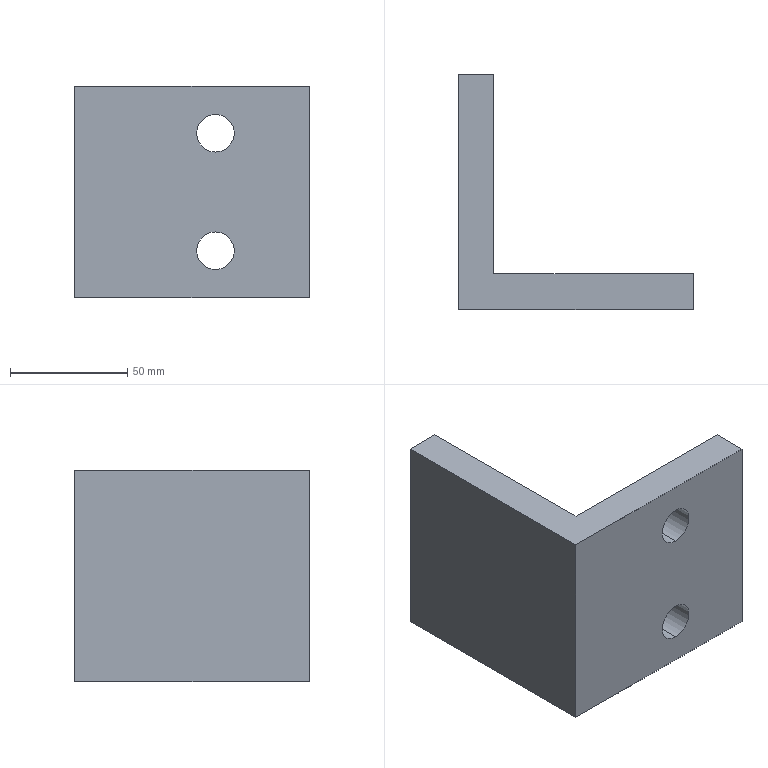Part | SolidWorks | features Extrusion 1, ICE 1 | 1 solid | 12 faces | box 100 x 100 x 90 mm | volume 243718 mm3 | plane 8 | cylinder 4 | commonest cylinder face diameters 16 x4
STEP:
#1=CARTESIAN_POINT('',(60.,0.,12.));
#2=VERTEX_POINT('',#1);
#3=CARTESIAN_POINT('',(60.,0.,28.));
#4=VERTEX_POINT('',#3);
#5=CARTESIAN_POINT('',(60.,0.,20.));
#6=DIRECTION('',(0.,1.,0.));
#7=DIRECTION('',(0.,0.,1.));
#8=AXIS2_PLACEMENT_3D('',#5,#6,#7);
#9=CIRCLE('',#8,8.);
#10=EDGE_CURVE('',#2,#4,#9,.T.);
#11=ORIENTED_EDGE('',*,*,#10,.F.);
#12=CARTESIAN_POINT('',(60.,15.,12.));
#13=VERTEX_POINT('',#12);
#14=CARTESIAN_POINT('',(60.,-75.,12.));
#15=DIRECTION('',(0.,1.,0.));
#16=VECTOR('',#15,1000.);
#17=LINE('',#14,#16);
#18=EDGE_CURVE('',#2,#13,#17,.T.);
#19=ORIENTED_EDGE('',*,*,#18,.T.);
#20=CARTESIAN_POINT('',(60.,15.,28.));
#21=VERTEX_POINT('',#20);
#22=CARTESIAN_POINT('',(60.,15.,20.));
#23=DIRECTION('',(0.,1.,0.));
#24=DIRECTION('',(0.,0.,1.));
#25=AXIS2_PLACEMENT_3D('',#22,#23,#24);
#26=CIRCLE('',#25,8.);
#27=EDGE_CURVE('',#13,#21,#26,.T.);
#28=ORIENTED_EDGE('',*,*,#27,.T.);
#29=CARTESIAN_POINT('',(60.,-75.,28.));
#30=DIRECTION('',(0.,1.,0.));
#31=VECTOR('',#30,1000.);
#32=LINE('',#29,#31);
#33=EDGE_CURVE('',#4,#21,#32,.T.);
#34=ORIENTED_EDGE('',*,*,#33,.F.);
#35=EDGE_LOOP('',(#11,#19,#28,#34));
#36=FACE_OUTER_BOUND('',#35,.T.);
#37=CARTESIAN_POINT('',(60.,-75.,20.));
#38=DIRECTION('',(0.,1.,0.));
#39=DIRECTION('',(0.,0.,1.));
#40=AXIS2_PLACEMENT_3D('',#37,#38,#39);
#41=CYLINDRICAL_SURFACE('',#40,8.);
#42=ADVANCED_FACE('',(#36),#41,.F.);
#43=CARTESIAN_POINT('',(60.,0.,62.));
#44=VERTEX_POINT('',#43);
#45=CARTESIAN_POINT('',(60.,0.,78.));
#46=VERTEX_POINT('',#45);
#47=CARTESIAN_POINT('',(60.,0.,70.));
#48=DIRECTION('',(0.,1.,0.));
#49=DIRECTION('',(0.,0.,1.));
#50=AXIS2_PLACEMENT_3D('',#47,#48,#49);
#51=CIRCLE('',#50,8.);
#52=EDGE_CURVE('',#44,#46,#51,.T.);
#53=ORIENTED_EDGE('',*,*,#52,.F.);
#54=CARTESIAN_POINT('',(60.,15.,62.));
#55=VERTEX_POINT('',#54);
#56=CARTESIAN_POINT('',(60.,-75.,62.));
#57=DIRECTION('',(0.,1.,0.));
#58=VECTOR('',#57,1000.);
#59=LINE('',#56,#58);
#60=EDGE_CURVE('',#44,#55,#59,.T.);
#61=ORIENTED_EDGE('',*,*,#60,.T.);
#62=CARTESIAN_POINT('',(60.,15.,78.));
#63=VERTEX_POINT('',#62);
#64=CARTESIAN_POINT('',(60.,15.,70.));
#65=DIRECTION('',(0.,1.,0.));
#66=DIRECTION('',(0.,0.,1.));
#67=AXIS2_PLACEMENT_3D('',#64,#65,#66);
#68=CIRCLE('',#67,8.);
#69=EDGE_CURVE('',#55,#63,#68,.T.);
#70=ORIENTED_EDGE('',*,*,#69,.T.);
#71=CARTESIAN_POINT('',(60.,-75.,78.));
#72=DIRECTION('',(0.,1.,0.));
#73=VECTOR('',#72,1000.);
#74=LINE('',#71,#73);
#75=EDGE_CURVE('',#46,#63,#74,.T.);
#76=ORIENTED_EDGE('',*,*,#75,.F.);
#77=EDGE_LOOP('',(#53,#61,#70,#76));
#78=FACE_OUTER_BOUND('',#77,.T.);
#79=CARTESIAN_POINT('',(60.,-75.,70.));
#80=DIRECTION('',(0.,1.,0.));
#81=DIRECTION('',(0.,0.,1.));
#82=AXIS2_PLACEMENT_3D('',#79,#80,#81);
#83=CYLINDRICAL_SURFACE('',#82,8.);
#84=ADVANCED_FACE('',(#78),#83,.F.);
#85=CARTESIAN_POINT('',(60.,0.,20.));
#86=DIRECTION('',(0.,1.,0.));
#87=DIRECTION('',(0.,0.,1.));
#88=AXIS2_PLACEMENT_3D('',#85,#86,#87);
#89=CIRCLE('',#88,8.);
#90=EDGE_CURVE('',#4,#2,#89,.T.);
#91=ORIENTED_EDGE('',*,*,#90,.T.);
#92=ORIENTED_EDGE('',*,*,#10,.T.);
#93=EDGE_LOOP('',(#91,#92));
#94=FACE_BOUND('',#93,.T.);
#95=CARTESIAN_POINT('',(60.,0.,70.));
#96=DIRECTION('',(0.,1.,0.));
#97=DIRECTION('',(0.,0.,1.));
#98=AXIS2_PLACEMENT_3D('',#95,#96,#97);
#99=CIRCLE('',#98,8.);
#100=EDGE_CURVE('',#46,#44,#99,.T.);
#101=ORIENTED_EDGE('',*,*,#100,.T.);
#102=ORIENTED_EDGE('',*,*,#52,.T.);
#103=EDGE_LOOP('',(#101,#102));
#104=FACE_BOUND('',#103,.T.);
#105=CARTESIAN_POINT('',(0.,0.,0.));
#106=VERTEX_POINT('',#105);
#107=CARTESIAN_POINT('',(100.,0.,0.));
#108=VERTEX_POINT('',#107);
#109=CARTESIAN_POINT('',(100.,0.,0.));
#110=DIRECTION('',(1.,0.,0.));
#111=VECTOR('',#110,1000.);
#112=LINE('',#109,#111);
#113=EDGE_CURVE('',#106,#108,#112,.T.);
#114=ORIENTED_EDGE('',*,*,#113,.T.);
#115=CARTESIAN_POINT('',(100.,0.,90.));
#116=VERTEX_POINT('',#115);
#117=CARTESIAN_POINT('',(100.,0.,90.));
#118=DIRECTION('',(0.,0.,-1.));
#119=VECTOR('',#118,1000.);
#120=LINE('',#117,#119);
#121=EDGE_CURVE('',#116,#108,#120,.T.);
#122=ORIENTED_EDGE('',*,*,#121,.F.);
#123=CARTESIAN_POINT('',(0.,0.,90.));
#124=VERTEX_POINT('',#123);
#125=CARTESIAN_POINT('',(100.,0.,90.));
#126=DIRECTION('',(1.,0.,0.));
#127=VECTOR('',#126,1000.);
#128=LINE('',#125,#127);
#129=EDGE_CURVE('',#124,#116,#128,.T.);
#130=ORIENTED_EDGE('',*,*,#129,.F.);
#131=CARTESIAN_POINT('',(0.,0.,90.));
#132=DIRECTION('',(0.,0.,-1.));
#133=VECTOR('',#132,1000.);
#134=LINE('',#131,#133);
#135=EDGE_CURVE('',#124,#106,#134,.T.);
#136=ORIENTED_EDGE('',*,*,#135,.T.);
#137=EDGE_LOOP('',(#114,#122,#130,#136));
#138=FACE_OUTER_BOUND('',#137,.T.);
#139=CARTESIAN_POINT('',(100.,0.,90.));
#140=DIRECTION('',(0.,1.,0.));
#141=DIRECTION('',(0.,0.,1.));
#142=AXIS2_PLACEMENT_3D('',#139,#140,#141);
#143=PLANE('',#142);
#144=ADVANCED_FACE('',(#94,#104,#138),#143,.F.);
#145=CARTESIAN_POINT('',(100.,15.,0.));
#146=VERTEX_POINT('',#145);
#147=CARTESIAN_POINT('',(100.,15.,0.));
#148=DIRECTION('',(0.,1.,0.));
#149=VECTOR('',#148,1000.);
#150=LINE('',#147,#149);
#151=EDGE_CURVE('',#108,#146,#150,.T.);
#152=ORIENTED_EDGE('',*,*,#151,.T.);
#153=CARTESIAN_POINT('',(100.,15.,90.));
#154=VERTEX_POINT('',#153);
#155=CARTESIAN_POINT('',(100.,15.,90.));
#156=DIRECTION('',(0.,0.,-1.));
#157=VECTOR('',#156,1000.);
#158=LINE('',#155,#157);
#159=EDGE_CURVE('',#154,#146,#158,.T.);
#160=ORIENTED_EDGE('',*,*,#159,.F.);
#161=CARTESIAN_POINT('',(100.,15.,90.));
#162=DIRECTION('',(0.,1.,0.));
#163=VECTOR('',#162,1000.);
#164=LINE('',#161,#163);
#165=EDGE_CURVE('',#116,#154,#164,.T.);
#166=ORIENTED_EDGE('',*,*,#165,.F.);
#167=ORIENTED_EDGE('',*,*,#121,.T.);
#168=EDGE_LOOP('',(#152,#160,#166,#167));
#169=FACE_OUTER_BOUND('',#168,.T.);
#170=CARTESIAN_POINT('',(100.,15.,90.));
#171=DIRECTION('',(-1.,0.,0.));
#172=DIRECTION('',(0.,0.,1.));
#173=AXIS2_PLACEMENT_3D('',#170,#171,#172);
#174=PLANE('',#173);
#175=ADVANCED_FACE('',(#169),#174,.F.);
#176=CARTESIAN_POINT('',(60.,15.,20.));
#177=DIRECTION('',(0.,1.,0.));
#178=DIRECTION('',(0.,0.,1.));
#179=AXIS2_PLACEMENT_3D('',#176,#177,#178);
#180=CIRCLE('',#179,8.);
#181=EDGE_CURVE('',#21,#13,#180,.T.);
#182=ORIENTED_EDGE('',*,*,#181,.F.);
#183=ORIENTED_EDGE('',*,*,#27,.F.);
#184=EDGE_LOOP('',(#182,#183));
#185=FACE_BOUND('',#184,.T.);
#186=CARTESIAN_POINT('',(60.,15.,70.));
#187=DIRECTION('',(0.,1.,0.));
#188=DIRECTION('',(0.,0.,1.));
#189=AXIS2_PLACEMENT_3D('',#186,#187,#188);
#190=CIRCLE('',#189,8.);
#191=EDGE_CURVE('',#63,#55,#190,.T.);
#192=ORIENTED_EDGE('',*,*,#191,.F.);
#193=ORIENTED_EDGE('',*,*,#69,.F.);
#194=EDGE_LOOP('',(#192,#193));
#195=FACE_BOUND('',#194,.T.);
#196=CARTESIAN_POINT('',(15.,15.,0.));
#197=VERTEX_POINT('',#196);
#198=CARTESIAN_POINT('',(15.,15.,0.));
#199=DIRECTION('',(-1.,0.,0.));
#200=VECTOR('',#199,1000.);
#201=LINE('',#198,#200);
#202=EDGE_CURVE('',#146,#197,#201,.T.);
#203=ORIENTED_EDGE('',*,*,#202,.T.);
#204=CARTESIAN_POINT('',(15.,15.,90.));
#205=VERTEX_POINT('',#204);
#206=CARTESIAN_POINT('',(15.,15.,90.));
#207=DIRECTION('',(0.,0.,-1.));
#208=VECTOR('',#207,1000.);
#209=LINE('',#206,#208);
#210=EDGE_CURVE('',#205,#197,#209,.T.);
#211=ORIENTED_EDGE('',*,*,#210,.F.);
#212=CARTESIAN_POINT('',(15.,15.,90.));
#213=DIRECTION('',(-1.,0.,0.));
#214=VECTOR('',#213,1000.);
#215=LINE('',#212,#214);
#216=EDGE_CURVE('',#154,#205,#215,.T.);
#217=ORIENTED_EDGE('',*,*,#216,.F.);
#218=ORIENTED_EDGE('',*,*,#159,.T.);
#219=EDGE_LOOP('',(#203,#211,#217,#218));
#220=FACE_OUTER_BOUND('',#219,.T.);
#221=CARTESIAN_POINT('',(15.,15.,90.));
#222=DIRECTION('',(0.,-1.,0.));
#223=DIRECTION('',(0.,0.,-1.));
#224=AXIS2_PLACEMENT_3D('',#221,#222,#223);
#225=PLANE('',#224);
#226=ADVANCED_FACE('',(#185,#195,#220),#225,.F.);
#227=CARTESIAN_POINT('',(15.,100.,0.));
#228=VERTEX_POINT('',#227);
#229=CARTESIAN_POINT('',(15.,100.,0.));
#230=DIRECTION('',(0.,1.,0.));
#231=VECTOR('',#230,1000.);
#232=LINE('',#229,#231);
#233=EDGE_CURVE('',#197,#228,#232,.T.);
#234=ORIENTED_EDGE('',*,*,#233,.T.);
#235=CARTESIAN_POINT('',(15.,100.,90.));
#236=VERTEX_POINT('',#235);
#237=CARTESIAN_POINT('',(15.,100.,90.));
#238=DIRECTION('',(0.,0.,-1.));
#239=VECTOR('',#238,1000.);
#240=LINE('',#237,#239);
#241=EDGE_CURVE('',#236,#228,#240,.T.);
#242=ORIENTED_EDGE('',*,*,#241,.F.);
#243=CARTESIAN_POINT('',(15.,100.,90.));
#244=DIRECTION('',(0.,1.,0.));
#245=VECTOR('',#244,1000.);
#246=LINE('',#243,#245);
#247=EDGE_CURVE('',#205,#236,#246,.T.);
#248=ORIENTED_EDGE('',*,*,#247,.F.);
#249=ORIENTED_EDGE('',*,*,#210,.T.);
#250=EDGE_LOOP('',(#234,#242,#248,#249));
#251=FACE_OUTER_BOUND('',#250,.T.);
#252=CARTESIAN_POINT('',(15.,100.,90.));
#253=DIRECTION('',(-1.,0.,0.));
#254=DIRECTION('',(0.,-1.,0.));
#255=AXIS2_PLACEMENT_3D('',#252,#253,#254);
#256=PLANE('',#255);
#257=ADVANCED_FACE('',(#251),#256,.F.);
#258=CARTESIAN_POINT('',(0.,100.,0.));
#259=VERTEX_POINT('',#258);
#260=CARTESIAN_POINT('',(0.,100.,0.));
#261=DIRECTION('',(-1.,0.,0.));
#262=VECTOR('',#261,1000.);
#263=LINE('',#260,#262);
#264=EDGE_CURVE('',#228,#259,#263,.T.);
#265=ORIENTED_EDGE('',*,*,#264,.T.);
#266=CARTESIAN_POINT('',(0.,100.,90.));
#267=VERTEX_POINT('',#266);
#268=CARTESIAN_POINT('',(0.,100.,90.));
#269=DIRECTION('',(0.,0.,-1.));
#270=VECTOR('',#269,1000.);
#271=LINE('',#268,#270);
#272=EDGE_CURVE('',#267,#259,#271,.T.);
#273=ORIENTED_EDGE('',*,*,#272,.F.);
#274=CARTESIAN_POINT('',(0.,100.,90.));
#275=DIRECTION('',(-1.,0.,0.));
#276=VECTOR('',#275,1000.);
#277=LINE('',#274,#276);
#278=EDGE_CURVE('',#236,#267,#277,.T.);
#279=ORIENTED_EDGE('',*,*,#278,.F.);
#280=ORIENTED_EDGE('',*,*,#241,.T.);
#281=EDGE_LOOP('',(#265,#273,#279,#280));
#282=FACE_OUTER_BOUND('',#281,.T.);
#283=CARTESIAN_POINT('',(0.,100.,90.));
#284=DIRECTION('',(0.,-1.,0.));
#285=DIRECTION('',(0.,0.,-1.));
#286=AXIS2_PLACEMENT_3D('',#283,#284,#285);
#287=PLANE('',#286);
#288=ADVANCED_FACE('',(#282),#287,.F.);
#289=CARTESIAN_POINT('',(0.,0.,0.));
#290=DIRECTION('',(0.,-1.,0.));
#291=VECTOR('',#290,1000.);
#292=LINE('',#289,#291);
#293=EDGE_CURVE('',#259,#106,#292,.T.);
#294=ORIENTED_EDGE('',*,*,#293,.T.);
#295=ORIENTED_EDGE('',*,*,#135,.F.);
#296=CARTESIAN_POINT('',(0.,0.,90.));
#297=DIRECTION('',(0.,-1.,0.));
#298=VECTOR('',#297,1000.);
#299=LINE('',#296,#298);
#300=EDGE_CURVE('',#267,#124,#299,.T.);
#301=ORIENTED_EDGE('',*,*,#300,.F.);
#302=ORIENTED_EDGE('',*,*,#272,.T.);
#303=EDGE_LOOP('',(#294,#295,#301,#302));
#304=FACE_OUTER_BOUND('',#303,.T.);
#305=CARTESIAN_POINT('',(0.,0.,90.));
#306=DIRECTION('',(1.,0.,0.));
#307=DIRECTION('',(0.,0.,-1.));
#308=AXIS2_PLACEMENT_3D('',#305,#306,#307);
#309=PLANE('',#308);
#310=ADVANCED_FACE('',(#304),#309,.F.);
#311=ORIENTED_EDGE('',*,*,#129,.T.);
#312=ORIENTED_EDGE('',*,*,#165,.T.);
#313=ORIENTED_EDGE('',*,*,#216,.T.);
#314=ORIENTED_EDGE('',*,*,#247,.T.);
#315=ORIENTED_EDGE('',*,*,#278,.T.);
#316=ORIENTED_EDGE('',*,*,#300,.T.);
#317=EDGE_LOOP('',(#311,#312,#313,#314,#315,#316));
#318=FACE_OUTER_BOUND('',#317,.T.);
#319=CARTESIAN_POINT('',(0.,0.,90.));
#320=DIRECTION('',(0.,0.,-1.));
#321=DIRECTION('',(-1.,0.,0.));
#322=AXIS2_PLACEMENT_3D('',#319,#320,#321);
#323=PLANE('',#322);
#324=ADVANCED_FACE('',(#318),#323,.F.);
#325=ORIENTED_EDGE('',*,*,#113,.F.);
#326=ORIENTED_EDGE('',*,*,#293,.F.);
#327=ORIENTED_EDGE('',*,*,#264,.F.);
#328=ORIENTED_EDGE('',*,*,#233,.F.);
#329=ORIENTED_EDGE('',*,*,#202,.F.);
#330=ORIENTED_EDGE('',*,*,#151,.F.);
#331=EDGE_LOOP('',(#325,#326,#327,#328,#329,#330));
#332=FACE_OUTER_BOUND('',#331,.T.);
#333=CARTESIAN_POINT('',(0.,0.,0.));
#334=DIRECTION('',(0.,0.,-1.));
#335=DIRECTION('',(-1.,0.,0.));
#336=AXIS2_PLACEMENT_3D('',#333,#334,#335);
#337=PLANE('',#336);
#338=ADVANCED_FACE('',(#332),#337,.T.);
#339=ORIENTED_EDGE('',*,*,#60,.F.);
#340=ORIENTED_EDGE('',*,*,#100,.F.);
#341=ORIENTED_EDGE('',*,*,#75,.T.);
#342=ORIENTED_EDGE('',*,*,#191,.T.);
#343=EDGE_LOOP('',(#339,#340,#341,#342));
#344=FACE_OUTER_BOUND('',#343,.T.);
#345=CARTESIAN_POINT('',(60.,-75.,70.));
#346=DIRECTION('',(0.,1.,0.));
#347=DIRECTION('',(0.,0.,1.));
#348=AXIS2_PLACEMENT_3D('',#345,#346,#347);
#349=CYLINDRICAL_SURFACE('',#348,8.);
#350=ADVANCED_FACE('',(#344),#349,.F.);
#351=ORIENTED_EDGE('',*,*,#18,.F.);
#352=ORIENTED_EDGE('',*,*,#90,.F.);
#353=ORIENTED_EDGE('',*,*,#33,.T.);
#354=ORIENTED_EDGE('',*,*,#181,.T.);
#355=EDGE_LOOP('',(#351,#352,#353,#354));
#356=FACE_OUTER_BOUND('',#355,.T.);
#357=CARTESIAN_POINT('',(60.,-75.,20.));
#358=DIRECTION('',(0.,1.,0.));
#359=DIRECTION('',(0.,0.,1.));
#360=AXIS2_PLACEMENT_3D('',#357,#358,#359);
#361=CYLINDRICAL_SURFACE('',#360,8.);
#362=ADVANCED_FACE('',(#356),#361,.F.);
#363=CLOSED_SHELL('',(#42,#84,#144,#175,#226,#257,#288,#310,#324,#338,#350,#362));
#364=MANIFOLD_SOLID_BREP('',#363);
#365=CARTESIAN_POINT('',(0.,0.,0.));
#366=DIRECTION('',(0.,0.,1.));
#367=DIRECTION('',(1.,0.,0.));
#368=AXIS2_PLACEMENT_3D('',#365,#366,#367);
#369=(LENGTH_UNIT()NAMED_UNIT(*)SI_UNIT(.MILLI.,.METRE.));
#370=UNCERTAINTY_MEASURE_WITH_UNIT(LENGTH_MEASURE(0.00001),#369,'','');
#371=(NAMED_UNIT(*)PLANE_ANGLE_UNIT()SI_UNIT($,.RADIAN.));
#372=(NAMED_UNIT(*)SI_UNIT($,.STERADIAN.)SOLID_ANGLE_UNIT());
#373=(GEOMETRIC_REPRESENTATION_CONTEXT(3)GLOBAL_UNCERTAINTY_ASSIGNED_CONTEXT((#370))GLOBAL_UNIT_ASSIGNED_CONTEXT((#369,#371,#372))REPRESENTATION_CONTEXT('',''));
#374=ADVANCED_BREP_SHAPE_REPRESENTATION('',(#364,#368),#373);